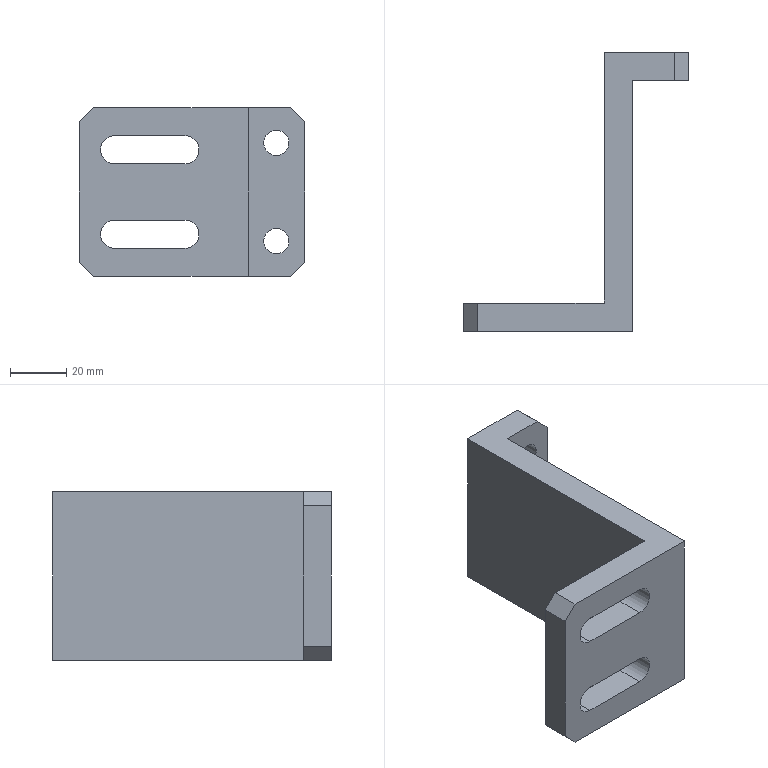Part | SolidWorks | features HoleWzd 2, Chamfer 1, Extrusion 1 | 1 solid | 26 faces | box 80 x 99 x 60 mm | volume 93057 mm3 | plane 18 | cylinder 8 | commonest cylinder face diameters 9 x4 10 x4
STEP:
#1=CARTESIAN_POINT('',(10.,89.,-22.));
#2=VERTEX_POINT('',#1);
#3=CARTESIAN_POINT('',(10.,89.,-13.));
#4=VERTEX_POINT('',#3);
#5=CARTESIAN_POINT('',(10.,89.,-17.5));
#6=DIRECTION('',(0.,1.,0.));
#7=DIRECTION('',(0.,0.,1.));
#8=AXIS2_PLACEMENT_3D('',#5,#6,#7);
#9=CIRCLE('',#8,4.5);
#10=EDGE_CURVE('',#2,#4,#9,.T.);
#11=ORIENTED_EDGE('',*,*,#10,.F.);
#12=CARTESIAN_POINT('',(10.,99.,-22.));
#13=VERTEX_POINT('',#12);
#14=CARTESIAN_POINT('',(10.,99.,-22.));
#15=DIRECTION('',(0.,1.,0.));
#16=VECTOR('',#15,1000.);
#17=LINE('',#14,#16);
#18=EDGE_CURVE('',#2,#13,#17,.T.);
#19=ORIENTED_EDGE('',*,*,#18,.T.);
#20=CARTESIAN_POINT('',(10.,99.,-13.));
#21=VERTEX_POINT('',#20);
#22=CARTESIAN_POINT('',(10.,99.,-17.5));
#23=DIRECTION('',(0.,1.,0.));
#24=DIRECTION('',(0.,0.,1.));
#25=AXIS2_PLACEMENT_3D('',#22,#23,#24);
#26=CIRCLE('',#25,4.5);
#27=EDGE_CURVE('',#13,#21,#26,.T.);
#28=ORIENTED_EDGE('',*,*,#27,.T.);
#29=CARTESIAN_POINT('',(10.,99.,-13.));
#30=DIRECTION('',(0.,1.,0.));
#31=VECTOR('',#30,1000.);
#32=LINE('',#29,#31);
#33=EDGE_CURVE('',#4,#21,#32,.T.);
#34=ORIENTED_EDGE('',*,*,#33,.F.);
#35=EDGE_LOOP('',(#11,#19,#28,#34));
#36=FACE_OUTER_BOUND('',#35,.T.);
#37=CARTESIAN_POINT('',(10.,99.,-17.5));
#38=DIRECTION('',(0.,1.,0.));
#39=DIRECTION('',(0.,0.,1.));
#40=AXIS2_PLACEMENT_3D('',#37,#38,#39);
#41=CYLINDRICAL_SURFACE('',#40,4.5);
#42=ADVANCED_FACE('',(#36),#41,.F.);
#43=CARTESIAN_POINT('',(10.,89.,13.));
#44=VERTEX_POINT('',#43);
#45=CARTESIAN_POINT('',(10.,89.,22.));
#46=VERTEX_POINT('',#45);
#47=CARTESIAN_POINT('',(10.,89.,17.5));
#48=DIRECTION('',(0.,1.,0.));
#49=DIRECTION('',(0.,0.,1.));
#50=AXIS2_PLACEMENT_3D('',#47,#48,#49);
#51=CIRCLE('',#50,4.5);
#52=EDGE_CURVE('',#44,#46,#51,.T.);
#53=ORIENTED_EDGE('',*,*,#52,.F.);
#54=CARTESIAN_POINT('',(10.,99.,13.));
#55=VERTEX_POINT('',#54);
#56=CARTESIAN_POINT('',(10.,99.,13.));
#57=DIRECTION('',(0.,1.,0.));
#58=VECTOR('',#57,1000.);
#59=LINE('',#56,#58);
#60=EDGE_CURVE('',#44,#55,#59,.T.);
#61=ORIENTED_EDGE('',*,*,#60,.T.);
#62=CARTESIAN_POINT('',(10.,99.,22.));
#63=VERTEX_POINT('',#62);
#64=CARTESIAN_POINT('',(10.,99.,17.5));
#65=DIRECTION('',(0.,1.,0.));
#66=DIRECTION('',(0.,0.,1.));
#67=AXIS2_PLACEMENT_3D('',#64,#65,#66);
#68=CIRCLE('',#67,4.5);
#69=EDGE_CURVE('',#55,#63,#68,.T.);
#70=ORIENTED_EDGE('',*,*,#69,.T.);
#71=CARTESIAN_POINT('',(10.,99.,22.));
#72=DIRECTION('',(0.,1.,0.));
#73=VECTOR('',#72,1000.);
#74=LINE('',#71,#73);
#75=EDGE_CURVE('',#46,#63,#74,.T.);
#76=ORIENTED_EDGE('',*,*,#75,.F.);
#77=EDGE_LOOP('',(#53,#61,#70,#76));
#78=FACE_OUTER_BOUND('',#77,.T.);
#79=CARTESIAN_POINT('',(10.,99.,17.5));
#80=DIRECTION('',(0.,1.,0.));
#81=DIRECTION('',(0.,0.,1.));
#82=AXIS2_PLACEMENT_3D('',#79,#80,#81);
#83=CYLINDRICAL_SURFACE('',#82,4.5);
#84=ADVANCED_FACE('',(#78),#83,.F.);
#85=CARTESIAN_POINT('',(10.,99.,17.5));
#86=DIRECTION('',(0.,1.,0.));
#87=DIRECTION('',(0.,0.,1.));
#88=AXIS2_PLACEMENT_3D('',#85,#86,#87);
#89=CIRCLE('',#88,4.5);
#90=EDGE_CURVE('',#63,#55,#89,.T.);
#91=ORIENTED_EDGE('',*,*,#90,.F.);
#92=ORIENTED_EDGE('',*,*,#69,.F.);
#93=EDGE_LOOP('',(#91,#92));
#94=FACE_BOUND('',#93,.T.);
#95=CARTESIAN_POINT('',(20.,99.,25.));
#96=VERTEX_POINT('',#95);
#97=CARTESIAN_POINT('',(20.,99.,-25.));
#98=VERTEX_POINT('',#97);
#99=CARTESIAN_POINT('',(20.,99.,30.));
#100=DIRECTION('',(0.,0.,-1.));
#101=VECTOR('',#100,1000.);
#102=LINE('',#99,#101);
#103=EDGE_CURVE('',#96,#98,#102,.T.);
#104=ORIENTED_EDGE('',*,*,#103,.T.);
#105=CARTESIAN_POINT('',(15.,99.,-30.));
#106=VERTEX_POINT('',#105);
#107=CARTESIAN_POINT('',(20.,99.,-25.));
#108=DIRECTION('',(-0.7071,0.,-0.7071));
#109=VECTOR('',#108,1000.);
#110=LINE('',#107,#109);
#111=EDGE_CURVE('',#98,#106,#110,.T.);
#112=ORIENTED_EDGE('',*,*,#111,.T.);
#113=CARTESIAN_POINT('',(-10.,99.,-30.));
#114=VERTEX_POINT('',#113);
#115=CARTESIAN_POINT('',(-10.,99.,-30.));
#116=DIRECTION('',(-1.,0.,0.));
#117=VECTOR('',#116,1000.);
#118=LINE('',#115,#117);
#119=EDGE_CURVE('',#106,#114,#118,.T.);
#120=ORIENTED_EDGE('',*,*,#119,.T.);
#121=CARTESIAN_POINT('',(-10.,99.,30.));
#122=VERTEX_POINT('',#121);
#123=CARTESIAN_POINT('',(-10.,99.,30.));
#124=DIRECTION('',(0.,0.,-1.));
#125=VECTOR('',#124,1000.);
#126=LINE('',#123,#125);
#127=EDGE_CURVE('',#122,#114,#126,.T.);
#128=ORIENTED_EDGE('',*,*,#127,.F.);
#129=CARTESIAN_POINT('',(15.,99.,30.));
#130=VERTEX_POINT('',#129);
#131=CARTESIAN_POINT('',(-10.,99.,30.));
#132=DIRECTION('',(-1.,0.,0.));
#133=VECTOR('',#132,1000.);
#134=LINE('',#131,#133);
#135=EDGE_CURVE('',#130,#122,#134,.T.);
#136=ORIENTED_EDGE('',*,*,#135,.F.);
#137=CARTESIAN_POINT('',(15.,99.,30.));
#138=DIRECTION('',(0.7071,0.,-0.7071));
#139=VECTOR('',#138,1000.);
#140=LINE('',#137,#139);
#141=EDGE_CURVE('',#130,#96,#140,.T.);
#142=ORIENTED_EDGE('',*,*,#141,.T.);
#143=EDGE_LOOP('',(#104,#112,#120,#128,#136,#142));
#144=FACE_OUTER_BOUND('',#143,.T.);
#145=CARTESIAN_POINT('',(10.,99.,-17.5));
#146=DIRECTION('',(0.,1.,0.));
#147=DIRECTION('',(0.,0.,1.));
#148=AXIS2_PLACEMENT_3D('',#145,#146,#147);
#149=CIRCLE('',#148,4.5);
#150=EDGE_CURVE('',#21,#13,#149,.T.);
#151=ORIENTED_EDGE('',*,*,#150,.F.);
#152=ORIENTED_EDGE('',*,*,#27,.F.);
#153=EDGE_LOOP('',(#151,#152));
#154=FACE_BOUND('',#153,.T.);
#155=CARTESIAN_POINT('',(-10.,99.,30.));
#156=DIRECTION('',(0.,-1.,0.));
#157=DIRECTION('',(0.,0.,-1.));
#158=AXIS2_PLACEMENT_3D('',#155,#156,#157);
#159=PLANE('',#158);
#160=ADVANCED_FACE('',(#94,#144,#154),#159,.F.);
#161=CARTESIAN_POINT('',(-47.5,0.,-10.));
#162=VERTEX_POINT('',#161);
#163=CARTESIAN_POINT('',(-22.5,0.,-10.));
#164=VERTEX_POINT('',#163);
#165=CARTESIAN_POINT('',(-47.5,0.,-10.));
#166=DIRECTION('',(1.,0.,0.));
#167=VECTOR('',#166,1000.);
#168=LINE('',#165,#167);
#169=EDGE_CURVE('',#162,#164,#168,.T.);
#170=ORIENTED_EDGE('',*,*,#169,.T.);
#171=CARTESIAN_POINT('',(-22.5,0.,-20.));
#172=VERTEX_POINT('',#171);
#173=CARTESIAN_POINT('',(-22.5,0.,-15.));
#174=DIRECTION('',(0.,1.,0.));
#175=DIRECTION('',(0.,0.,1.));
#176=AXIS2_PLACEMENT_3D('',#173,#174,#175);
#177=CIRCLE('',#176,5.);
#178=EDGE_CURVE('',#164,#172,#177,.T.);
#179=ORIENTED_EDGE('',*,*,#178,.T.);
#180=CARTESIAN_POINT('',(-47.5,0.,-20.));
#181=VERTEX_POINT('',#180);
#182=CARTESIAN_POINT('',(-47.5,0.,-20.));
#183=DIRECTION('',(1.,0.,0.));
#184=VECTOR('',#183,1000.);
#185=LINE('',#182,#184);
#186=EDGE_CURVE('',#181,#172,#185,.T.);
#187=ORIENTED_EDGE('',*,*,#186,.F.);
#188=CARTESIAN_POINT('',(-47.5,0.,-15.));
#189=DIRECTION('',(0.,1.,0.));
#190=DIRECTION('',(0.,0.,1.));
#191=AXIS2_PLACEMENT_3D('',#188,#189,#190);
#192=CIRCLE('',#191,5.);
#193=EDGE_CURVE('',#181,#162,#192,.T.);
#194=ORIENTED_EDGE('',*,*,#193,.T.);
#195=EDGE_LOOP('',(#170,#179,#187,#194));
#196=FACE_BOUND('',#195,.T.);
#197=CARTESIAN_POINT('',(-47.5,0.,20.));
#198=VERTEX_POINT('',#197);
#199=CARTESIAN_POINT('',(-22.5,0.,20.));
#200=VERTEX_POINT('',#199);
#201=CARTESIAN_POINT('',(-47.5,0.,20.));
#202=DIRECTION('',(1.,0.,0.));
#203=VECTOR('',#202,1000.);
#204=LINE('',#201,#203);
#205=EDGE_CURVE('',#198,#200,#204,.T.);
#206=ORIENTED_EDGE('',*,*,#205,.T.);
#207=CARTESIAN_POINT('',(-22.5,0.,10.));
#208=VERTEX_POINT('',#207);
#209=CARTESIAN_POINT('',(-22.5,0.,15.));
#210=DIRECTION('',(0.,1.,0.));
#211=DIRECTION('',(0.,0.,1.));
#212=AXIS2_PLACEMENT_3D('',#209,#210,#211);
#213=CIRCLE('',#212,5.);
#214=EDGE_CURVE('',#200,#208,#213,.T.);
#215=ORIENTED_EDGE('',*,*,#214,.T.);
#216=CARTESIAN_POINT('',(-47.5,0.,10.));
#217=VERTEX_POINT('',#216);
#218=CARTESIAN_POINT('',(-47.5,0.,10.));
#219=DIRECTION('',(1.,0.,0.));
#220=VECTOR('',#219,1000.);
#221=LINE('',#218,#220);
#222=EDGE_CURVE('',#217,#208,#221,.T.);
#223=ORIENTED_EDGE('',*,*,#222,.F.);
#224=CARTESIAN_POINT('',(-47.5,0.,15.));
#225=DIRECTION('',(0.,1.,0.));
#226=DIRECTION('',(0.,0.,1.));
#227=AXIS2_PLACEMENT_3D('',#224,#225,#226);
#228=CIRCLE('',#227,5.);
#229=EDGE_CURVE('',#217,#198,#228,.T.);
#230=ORIENTED_EDGE('',*,*,#229,.T.);
#231=EDGE_LOOP('',(#206,#215,#223,#230));
#232=FACE_BOUND('',#231,.T.);
#233=CARTESIAN_POINT('',(-60.,0.,25.));
#234=VERTEX_POINT('',#233);
#235=CARTESIAN_POINT('',(-60.,0.,-25.));
#236=VERTEX_POINT('',#235);
#237=CARTESIAN_POINT('',(-60.,0.,30.));
#238=DIRECTION('',(0.,0.,-1.));
#239=VECTOR('',#238,1000.);
#240=LINE('',#237,#239);
#241=EDGE_CURVE('',#234,#236,#240,.T.);
#242=ORIENTED_EDGE('',*,*,#241,.T.);
#243=CARTESIAN_POINT('',(-55.,0.,-30.));
#244=VERTEX_POINT('',#243);
#245=CARTESIAN_POINT('',(-60.,0.,-25.));
#246=DIRECTION('',(0.7071,0.,-0.7071));
#247=VECTOR('',#246,1000.);
#248=LINE('',#245,#247);
#249=EDGE_CURVE('',#236,#244,#248,.T.);
#250=ORIENTED_EDGE('',*,*,#249,.T.);
#251=CARTESIAN_POINT('',(0.,0.,-30.));
#252=VERTEX_POINT('',#251);
#253=CARTESIAN_POINT('',(0.,0.,-30.));
#254=DIRECTION('',(1.,0.,0.));
#255=VECTOR('',#254,1000.);
#256=LINE('',#253,#255);
#257=EDGE_CURVE('',#244,#252,#256,.T.);
#258=ORIENTED_EDGE('',*,*,#257,.T.);
#259=CARTESIAN_POINT('',(0.,0.,30.));
#260=VERTEX_POINT('',#259);
#261=CARTESIAN_POINT('',(0.,0.,30.));
#262=DIRECTION('',(0.,0.,-1.));
#263=VECTOR('',#262,1000.);
#264=LINE('',#261,#263);
#265=EDGE_CURVE('',#260,#252,#264,.T.);
#266=ORIENTED_EDGE('',*,*,#265,.F.);
#267=CARTESIAN_POINT('',(-55.,0.,30.));
#268=VERTEX_POINT('',#267);
#269=CARTESIAN_POINT('',(0.,0.,30.));
#270=DIRECTION('',(1.,0.,0.));
#271=VECTOR('',#270,1000.);
#272=LINE('',#269,#271);
#273=EDGE_CURVE('',#268,#260,#272,.T.);
#274=ORIENTED_EDGE('',*,*,#273,.F.);
#275=CARTESIAN_POINT('',(-55.,0.,30.));
#276=DIRECTION('',(-0.7071,0.,-0.7071));
#277=VECTOR('',#276,1000.);
#278=LINE('',#275,#277);
#279=EDGE_CURVE('',#268,#234,#278,.T.);
#280=ORIENTED_EDGE('',*,*,#279,.T.);
#281=EDGE_LOOP('',(#242,#250,#258,#266,#274,#280));
#282=FACE_OUTER_BOUND('',#281,.T.);
#283=CARTESIAN_POINT('',(0.,0.,30.));
#284=DIRECTION('',(0.,1.,0.));
#285=DIRECTION('',(-1.,0.,0.));
#286=AXIS2_PLACEMENT_3D('',#283,#284,#285);
#287=PLANE('',#286);
#288=ADVANCED_FACE('',(#196,#232,#282),#287,.F.);
#289=CARTESIAN_POINT('',(0.,89.,-30.));
#290=VERTEX_POINT('',#289);
#291=CARTESIAN_POINT('',(0.,0.,-30.));
#292=DIRECTION('',(0.,1.,0.));
#293=VECTOR('',#292,1000.);
#294=LINE('',#291,#293);
#295=EDGE_CURVE('',#252,#290,#294,.T.);
#296=ORIENTED_EDGE('',*,*,#295,.T.);
#297=CARTESIAN_POINT('',(0.,89.,30.));
#298=VERTEX_POINT('',#297);
#299=CARTESIAN_POINT('',(0.,89.,30.));
#300=DIRECTION('',(0.,0.,-1.));
#301=VECTOR('',#300,1000.);
#302=LINE('',#299,#301);
#303=EDGE_CURVE('',#298,#290,#302,.T.);
#304=ORIENTED_EDGE('',*,*,#303,.F.);
#305=CARTESIAN_POINT('',(0.,0.,30.));
#306=DIRECTION('',(0.,1.,0.));
#307=VECTOR('',#306,1000.);
#308=LINE('',#305,#307);
#309=EDGE_CURVE('',#260,#298,#308,.T.);
#310=ORIENTED_EDGE('',*,*,#309,.F.);
#311=ORIENTED_EDGE('',*,*,#265,.T.);
#312=EDGE_LOOP('',(#296,#304,#310,#311));
#313=FACE_OUTER_BOUND('',#312,.T.);
#314=CARTESIAN_POINT('',(0.,0.,30.));
#315=DIRECTION('',(-1.,0.,0.));
#316=DIRECTION('',(0.,0.,1.));
#317=AXIS2_PLACEMENT_3D('',#314,#315,#316);
#318=PLANE('',#317);
#319=ADVANCED_FACE('',(#313),#318,.F.);
#320=CARTESIAN_POINT('',(10.,89.,-17.5));
#321=DIRECTION('',(0.,1.,0.));
#322=DIRECTION('',(0.,0.,1.));
#323=AXIS2_PLACEMENT_3D('',#320,#321,#322);
#324=CIRCLE('',#323,4.5);
#325=EDGE_CURVE('',#4,#2,#324,.T.);
#326=ORIENTED_EDGE('',*,*,#325,.T.);
#327=ORIENTED_EDGE('',*,*,#10,.T.);
#328=EDGE_LOOP('',(#326,#327));
#329=FACE_BOUND('',#328,.T.);
#330=CARTESIAN_POINT('',(10.,89.,17.5));
#331=DIRECTION('',(0.,1.,0.));
#332=DIRECTION('',(0.,0.,1.));
#333=AXIS2_PLACEMENT_3D('',#330,#331,#332);
#334=CIRCLE('',#333,4.5);
#335=EDGE_CURVE('',#46,#44,#334,.T.);
#336=ORIENTED_EDGE('',*,*,#335,.T.);
#337=ORIENTED_EDGE('',*,*,#52,.T.);
#338=EDGE_LOOP('',(#336,#337));
#339=FACE_BOUND('',#338,.T.);
#340=CARTESIAN_POINT('',(15.,89.,-30.));
#341=VERTEX_POINT('',#340);
#342=CARTESIAN_POINT('',(0.,89.,-30.));
#343=DIRECTION('',(1.,0.,0.));
#344=VECTOR('',#343,1000.);
#345=LINE('',#342,#344);
#346=EDGE_CURVE('',#290,#341,#345,.T.);
#347=ORIENTED_EDGE('',*,*,#346,.T.);
#348=CARTESIAN_POINT('',(20.,89.,-25.));
#349=VERTEX_POINT('',#348);
#350=CARTESIAN_POINT('',(20.,89.,-25.));
#351=DIRECTION('',(0.7071,0.,0.7071));
#352=VECTOR('',#351,1000.);
#353=LINE('',#350,#352);
#354=EDGE_CURVE('',#341,#349,#353,.T.);
#355=ORIENTED_EDGE('',*,*,#354,.T.);
#356=CARTESIAN_POINT('',(20.,89.,25.));
#357=VERTEX_POINT('',#356);
#358=CARTESIAN_POINT('',(20.,89.,30.));
#359=DIRECTION('',(0.,0.,-1.));
#360=VECTOR('',#359,1000.);
#361=LINE('',#358,#360);
#362=EDGE_CURVE('',#357,#349,#361,.T.);
#363=ORIENTED_EDGE('',*,*,#362,.F.);
#364=CARTESIAN_POINT('',(15.,89.,30.));
#365=VERTEX_POINT('',#364);
#366=CARTESIAN_POINT('',(15.,89.,30.));
#367=DIRECTION('',(-0.7071,0.,0.7071));
#368=VECTOR('',#367,1000.);
#369=LINE('',#366,#368);
#370=EDGE_CURVE('',#357,#365,#369,.T.);
#371=ORIENTED_EDGE('',*,*,#370,.T.);
#372=CARTESIAN_POINT('',(0.,89.,30.));
#373=DIRECTION('',(1.,0.,0.));
#374=VECTOR('',#373,1000.);
#375=LINE('',#372,#374);
#376=EDGE_CURVE('',#298,#365,#375,.T.);
#377=ORIENTED_EDGE('',*,*,#376,.F.);
#378=ORIENTED_EDGE('',*,*,#303,.T.);
#379=EDGE_LOOP('',(#347,#355,#363,#371,#377,#378));
#380=FACE_OUTER_BOUND('',#379,.T.);
#381=CARTESIAN_POINT('',(0.,89.,30.));
#382=DIRECTION('',(0.,1.,0.));
#383=DIRECTION('',(0.,0.,1.));
#384=AXIS2_PLACEMENT_3D('',#381,#382,#383);
#385=PLANE('',#384);
#386=ADVANCED_FACE('',(#329,#339,#380),#385,.F.);
#387=ORIENTED_EDGE('',*,*,#362,.T.);
#388=CARTESIAN_POINT('',(20.,99.,-25.));
#389=DIRECTION('',(0.,1.,0.));
#390=VECTOR('',#389,1000.);
#391=LINE('',#388,#390);
#392=EDGE_CURVE('',#349,#98,#391,.T.);
#393=ORIENTED_EDGE('',*,*,#392,.T.);
#394=ORIENTED_EDGE('',*,*,#103,.F.);
#395=CARTESIAN_POINT('',(20.,89.,25.));
#396=DIRECTION('',(0.,-1.,0.));
#397=VECTOR('',#396,1000.);
#398=LINE('',#395,#397);
#399=EDGE_CURVE('',#96,#357,#398,.T.);
#400=ORIENTED_EDGE('',*,*,#399,.T.);
#401=EDGE_LOOP('',(#387,#393,#394,#400));
#402=FACE_OUTER_BOUND('',#401,.T.);
#403=CARTESIAN_POINT('',(20.,99.,30.));
#404=DIRECTION('',(-1.,0.,0.));
#405=DIRECTION('',(0.,0.,1.));
#406=AXIS2_PLACEMENT_3D('',#403,#404,#405);
#407=PLANE('',#406);
#408=ADVANCED_FACE('',(#402),#407,.F.);
#409=CARTESIAN_POINT('',(-10.,10.,-30.));
#410=VERTEX_POINT('',#409);
#411=CARTESIAN_POINT('',(-10.,10.,-30.));
#412=DIRECTION('',(0.,-1.,0.));
#413=VECTOR('',#412,1000.);
#414=LINE('',#411,#413);
#415=EDGE_CURVE('',#114,#410,#414,.T.);
#416=ORIENTED_EDGE('',*,*,#415,.T.);
#417=CARTESIAN_POINT('',(-10.,10.,30.));
#418=VERTEX_POINT('',#417);
#419=CARTESIAN_POINT('',(-10.,10.,30.));
#420=DIRECTION('',(0.,0.,-1.));
#421=VECTOR('',#420,1000.);
#422=LINE('',#419,#421);
#423=EDGE_CURVE('',#418,#410,#422,.T.);
#424=ORIENTED_EDGE('',*,*,#423,.F.);
#425=CARTESIAN_POINT('',(-10.,10.,30.));
#426=DIRECTION('',(0.,-1.,0.));
#427=VECTOR('',#426,1000.);
#428=LINE('',#425,#427);
#429=EDGE_CURVE('',#122,#418,#428,.T.);
#430=ORIENTED_EDGE('',*,*,#429,.F.);
#431=ORIENTED_EDGE('',*,*,#127,.T.);
#432=EDGE_LOOP('',(#416,#424,#430,#431));
#433=FACE_OUTER_BOUND('',#432,.T.);
#434=CARTESIAN_POINT('',(-10.,10.,30.));
#435=DIRECTION('',(1.,0.,0.));
#436=DIRECTION('',(0.,0.,-1.));
#437=AXIS2_PLACEMENT_3D('',#434,#435,#436);
#438=PLANE('',#437);
#439=ADVANCED_FACE('',(#433),#438,.F.);
#440=CARTESIAN_POINT('',(-47.5,10.,-20.));
#441=VERTEX_POINT('',#440);
#442=CARTESIAN_POINT('',(-47.5,10.,-10.));
#443=VERTEX_POINT('',#442);
#444=CARTESIAN_POINT('',(-47.5,10.,-15.));
#445=DIRECTION('',(0.,1.,0.));
#446=DIRECTION('',(0.,0.,1.));
#447=AXIS2_PLACEMENT_3D('',#444,#445,#446);
#448=CIRCLE('',#447,5.);
#449=EDGE_CURVE('',#441,#443,#448,.T.);
#450=ORIENTED_EDGE('',*,*,#449,.F.);
#451=CARTESIAN_POINT('',(-22.5,10.,-20.));
#452=VERTEX_POINT('',#451);
#453=CARTESIAN_POINT('',(-47.5,10.,-20.));
#454=DIRECTION('',(1.,0.,0.));
#455=VECTOR('',#454,1000.);
#456=LINE('',#453,#455);
#457=EDGE_CURVE('',#441,#452,#456,.T.);
#458=ORIENTED_EDGE('',*,*,#457,.T.);
#459=CARTESIAN_POINT('',(-22.5,10.,-10.));
#460=VERTEX_POINT('',#459);
#461=CARTESIAN_POINT('',(-22.5,10.,-15.));
#462=DIRECTION('',(0.,1.,0.));
#463=DIRECTION('',(0.,0.,1.));
#464=AXIS2_PLACEMENT_3D('',#461,#462,#463);
#465=CIRCLE('',#464,5.);
#466=EDGE_CURVE('',#460,#452,#465,.T.);
#467=ORIENTED_EDGE('',*,*,#466,.F.);
#468=CARTESIAN_POINT('',(-47.5,10.,-10.));
#469=DIRECTION('',(1.,0.,0.));
#470=VECTOR('',#469,1000.);
#471=LINE('',#468,#470);
#472=EDGE_CURVE('',#443,#460,#471,.T.);
#473=ORIENTED_EDGE('',*,*,#472,.F.);
#474=EDGE_LOOP('',(#450,#458,#467,#473));
#475=FACE_BOUND('',#474,.T.);
#476=CARTESIAN_POINT('',(-47.5,10.,10.));
#477=VERTEX_POINT('',#476);
#478=CARTESIAN_POINT('',(-47.5,10.,20.));
#479=VERTEX_POINT('',#478);
#480=CARTESIAN_POINT('',(-47.5,10.,15.));
#481=DIRECTION('',(0.,1.,0.));
#482=DIRECTION('',(0.,0.,1.));
#483=AXIS2_PLACEMENT_3D('',#480,#481,#482);
#484=CIRCLE('',#483,5.);
#485=EDGE_CURVE('',#477,#479,#484,.T.);
#486=ORIENTED_EDGE('',*,*,#485,.F.);
#487=CARTESIAN_POINT('',(-22.5,10.,10.));
#488=VERTEX_POINT('',#487);
#489=CARTESIAN_POINT('',(-47.5,10.,10.));
#490=DIRECTION('',(1.,0.,0.));
#491=VECTOR('',#490,1000.);
#492=LINE('',#489,#491);
#493=EDGE_CURVE('',#477,#488,#492,.T.);
#494=ORIENTED_EDGE('',*,*,#493,.T.);
#495=CARTESIAN_POINT('',(-22.5,10.,20.));
#496=VERTEX_POINT('',#495);
#497=CARTESIAN_POINT('',(-22.5,10.,15.));
#498=DIRECTION('',(0.,1.,0.));
#499=DIRECTION('',(0.,0.,1.));
#500=AXIS2_PLACEMENT_3D('',#497,#498,#499);
#501=CIRCLE('',#500,5.);
#502=EDGE_CURVE('',#496,#488,#501,.T.);
#503=ORIENTED_EDGE('',*,*,#502,.F.);
#504=CARTESIAN_POINT('',(-47.5,10.,20.));
#505=DIRECTION('',(1.,0.,0.));
#506=VECTOR('',#505,1000.);
#507=LINE('',#504,#506);
#508=EDGE_CURVE('',#479,#496,#507,.T.);
#509=ORIENTED_EDGE('',*,*,#508,.F.);
#510=EDGE_LOOP('',(#486,#494,#503,#509));
#511=FACE_BOUND('',#510,.T.);
#512=CARTESIAN_POINT('',(-55.,10.,-30.));
#513=VERTEX_POINT('',#512);
#514=CARTESIAN_POINT('',(-10.,10.,-30.));
#515=DIRECTION('',(-1.,0.,0.));
#516=VECTOR('',#515,1000.);
#517=LINE('',#514,#516);
#518=EDGE_CURVE('',#410,#513,#517,.T.);
#519=ORIENTED_EDGE('',*,*,#518,.T.);
#520=CARTESIAN_POINT('',(-60.,10.,-25.));
#521=VERTEX_POINT('',#520);
#522=CARTESIAN_POINT('',(-60.,10.,-25.));
#523=DIRECTION('',(-0.7071,0.,0.7071));
#524=VECTOR('',#523,1000.);
#525=LINE('',#522,#524);
#526=EDGE_CURVE('',#513,#521,#525,.T.);
#527=ORIENTED_EDGE('',*,*,#526,.T.);
#528=CARTESIAN_POINT('',(-60.,10.,25.));
#529=VERTEX_POINT('',#528);
#530=CARTESIAN_POINT('',(-60.,10.,30.));
#531=DIRECTION('',(0.,0.,-1.));
#532=VECTOR('',#531,1000.);
#533=LINE('',#530,#532);
#534=EDGE_CURVE('',#529,#521,#533,.T.);
#535=ORIENTED_EDGE('',*,*,#534,.F.);
#536=CARTESIAN_POINT('',(-55.,10.,30.));
#537=VERTEX_POINT('',#536);
#538=CARTESIAN_POINT('',(-55.,10.,30.));
#539=DIRECTION('',(0.7071,0.,0.7071));
#540=VECTOR('',#539,1000.);
#541=LINE('',#538,#540);
#542=EDGE_CURVE('',#529,#537,#541,.T.);
#543=ORIENTED_EDGE('',*,*,#542,.T.);
#544=CARTESIAN_POINT('',(-10.,10.,30.));
#545=DIRECTION('',(-1.,0.,0.));
#546=VECTOR('',#545,1000.);
#547=LINE('',#544,#546);
#548=EDGE_CURVE('',#418,#537,#547,.T.);
#549=ORIENTED_EDGE('',*,*,#548,.F.);
#550=ORIENTED_EDGE('',*,*,#423,.T.);
#551=EDGE_LOOP('',(#519,#527,#535,#543,#549,#550));
#552=FACE_OUTER_BOUND('',#551,.T.);
#553=CARTESIAN_POINT('',(-10.,10.,30.));
#554=DIRECTION('',(0.,-1.,0.));
#555=DIRECTION('',(1.,0.,0.));
#556=AXIS2_PLACEMENT_3D('',#553,#554,#555);
#557=PLANE('',#556);
#558=ADVANCED_FACE('',(#475,#511,#552),#557,.F.);
#559=ORIENTED_EDGE('',*,*,#534,.T.);
#560=CARTESIAN_POINT('',(-60.,10.,-25.));
#561=DIRECTION('',(0.,-1.,0.));
#562=VECTOR('',#561,1000.);
#563=LINE('',#560,#562);
#564=EDGE_CURVE('',#521,#236,#563,.T.);
#565=ORIENTED_EDGE('',*,*,#564,.T.);
#566=ORIENTED_EDGE('',*,*,#241,.F.);
#567=CARTESIAN_POINT('',(-60.,10.,25.));
#568=DIRECTION('',(0.,1.,0.));
#569=VECTOR('',#568,1000.);
#570=LINE('',#567,#569);
#571=EDGE_CURVE('',#234,#529,#570,.T.);
#572=ORIENTED_EDGE('',*,*,#571,.T.);
#573=EDGE_LOOP('',(#559,#565,#566,#572));
#574=FACE_OUTER_BOUND('',#573,.T.);
#575=CARTESIAN_POINT('',(-60.,10.,30.));
#576=DIRECTION('',(1.,0.,0.));
#577=DIRECTION('',(0.,0.,-1.));
#578=AXIS2_PLACEMENT_3D('',#575,#576,#577);
#579=PLANE('',#578);
#580=ADVANCED_FACE('',(#574),#579,.F.);
#581=ORIENTED_EDGE('',*,*,#548,.T.);
#582=CARTESIAN_POINT('',(-55.,0.,30.));
#583=DIRECTION('',(0.,-1.,0.));
#584=VECTOR('',#583,1000.);
#585=LINE('',#582,#584);
#586=EDGE_CURVE('',#537,#268,#585,.T.);
#587=ORIENTED_EDGE('',*,*,#586,.T.);
#588=ORIENTED_EDGE('',*,*,#273,.T.);
#589=ORIENTED_EDGE('',*,*,#309,.T.);
#590=ORIENTED_EDGE('',*,*,#376,.T.);
#591=CARTESIAN_POINT('',(15.,99.,30.));
#592=DIRECTION('',(0.,1.,0.));
#593=VECTOR('',#592,1000.);
#594=LINE('',#591,#593);
#595=EDGE_CURVE('',#365,#130,#594,.T.);
#596=ORIENTED_EDGE('',*,*,#595,.T.);
#597=ORIENTED_EDGE('',*,*,#135,.T.);
#598=ORIENTED_EDGE('',*,*,#429,.T.);
#599=EDGE_LOOP('',(#581,#587,#588,#589,#590,#596,#597,#598));
#600=FACE_OUTER_BOUND('',#599,.T.);
#601=CARTESIAN_POINT('',(0.,0.,30.));
#602=DIRECTION('',(0.,0.,1.));
#603=DIRECTION('',(1.,0.,0.));
#604=AXIS2_PLACEMENT_3D('',#601,#602,#603);
#605=PLANE('',#604);
#606=ADVANCED_FACE('',(#600),#605,.T.);
#607=ORIENTED_EDGE('',*,*,#257,.F.);
#608=CARTESIAN_POINT('',(-55.,0.,-30.));
#609=DIRECTION('',(0.,1.,0.));
#610=VECTOR('',#609,1000.);
#611=LINE('',#608,#610);
#612=EDGE_CURVE('',#244,#513,#611,.T.);
#613=ORIENTED_EDGE('',*,*,#612,.T.);
#614=ORIENTED_EDGE('',*,*,#518,.F.);
#615=ORIENTED_EDGE('',*,*,#415,.F.);
#616=ORIENTED_EDGE('',*,*,#119,.F.);
#617=CARTESIAN_POINT('',(15.,0.,-30.));
#618=DIRECTION('',(0.,-1.,0.));
#619=VECTOR('',#618,1000.);
#620=LINE('',#617,#619);
#621=EDGE_CURVE('',#106,#341,#620,.T.);
#622=ORIENTED_EDGE('',*,*,#621,.T.);
#623=ORIENTED_EDGE('',*,*,#346,.F.);
#624=ORIENTED_EDGE('',*,*,#295,.F.);
#625=EDGE_LOOP('',(#607,#613,#614,#615,#616,#622,#623,#624));
#626=FACE_OUTER_BOUND('',#625,.T.);
#627=CARTESIAN_POINT('',(0.,0.,-30.));
#628=DIRECTION('',(0.,0.,1.));
#629=DIRECTION('',(1.,0.,0.));
#630=AXIS2_PLACEMENT_3D('',#627,#628,#629);
#631=PLANE('',#630);
#632=ADVANCED_FACE('',(#626),#631,.F.);
#633=ORIENTED_EDGE('',*,*,#60,.F.);
#634=ORIENTED_EDGE('',*,*,#335,.F.);
#635=ORIENTED_EDGE('',*,*,#75,.T.);
#636=ORIENTED_EDGE('',*,*,#90,.T.);
#637=EDGE_LOOP('',(#633,#634,#635,#636));
#638=FACE_OUTER_BOUND('',#637,.T.);
#639=CARTESIAN_POINT('',(10.,99.,17.5));
#640=DIRECTION('',(0.,1.,0.));
#641=DIRECTION('',(0.,0.,1.));
#642=AXIS2_PLACEMENT_3D('',#639,#640,#641);
#643=CYLINDRICAL_SURFACE('',#642,4.5);
#644=ADVANCED_FACE('',(#638),#643,.F.);
#645=ORIENTED_EDGE('',*,*,#18,.F.);
#646=ORIENTED_EDGE('',*,*,#325,.F.);
#647=ORIENTED_EDGE('',*,*,#33,.T.);
#648=ORIENTED_EDGE('',*,*,#150,.T.);
#649=EDGE_LOOP('',(#645,#646,#647,#648));
#650=FACE_OUTER_BOUND('',#649,.T.);
#651=CARTESIAN_POINT('',(10.,99.,-17.5));
#652=DIRECTION('',(0.,1.,0.));
#653=DIRECTION('',(0.,0.,1.));
#654=AXIS2_PLACEMENT_3D('',#651,#652,#653);
#655=CYLINDRICAL_SURFACE('',#654,4.5);
#656=ADVANCED_FACE('',(#650),#655,.F.);
#657=ORIENTED_EDGE('',*,*,#214,.F.);
#658=CARTESIAN_POINT('',(-22.5,10.,20.));
#659=DIRECTION('',(0.,-1.,0.));
#660=VECTOR('',#659,1000.);
#661=LINE('',#658,#660);
#662=EDGE_CURVE('',#496,#200,#661,.T.);
#663=ORIENTED_EDGE('',*,*,#662,.F.);
#664=ORIENTED_EDGE('',*,*,#502,.T.);
#665=CARTESIAN_POINT('',(-22.5,10.,10.));
#666=DIRECTION('',(0.,1.,0.));
#667=VECTOR('',#666,1000.);
#668=LINE('',#665,#667);
#669=EDGE_CURVE('',#208,#488,#668,.T.);
#670=ORIENTED_EDGE('',*,*,#669,.F.);
#671=EDGE_LOOP('',(#657,#663,#664,#670));
#672=FACE_OUTER_BOUND('',#671,.T.);
#673=CARTESIAN_POINT('',(-22.5,10.,15.));
#674=DIRECTION('',(0.,1.,0.));
#675=DIRECTION('',(0.,0.,1.));
#676=AXIS2_PLACEMENT_3D('',#673,#674,#675);
#677=CYLINDRICAL_SURFACE('',#676,5.);
#678=ADVANCED_FACE('',(#672),#677,.F.);
#679=ORIENTED_EDGE('',*,*,#485,.T.);
#680=CARTESIAN_POINT('',(-47.5,10.,20.));
#681=DIRECTION('',(0.,1.,0.));
#682=VECTOR('',#681,1000.);
#683=LINE('',#680,#682);
#684=EDGE_CURVE('',#198,#479,#683,.T.);
#685=ORIENTED_EDGE('',*,*,#684,.F.);
#686=ORIENTED_EDGE('',*,*,#229,.F.);
#687=CARTESIAN_POINT('',(-47.5,10.,10.));
#688=DIRECTION('',(0.,-1.,0.));
#689=VECTOR('',#688,1000.);
#690=LINE('',#687,#689);
#691=EDGE_CURVE('',#477,#217,#690,.T.);
#692=ORIENTED_EDGE('',*,*,#691,.F.);
#693=EDGE_LOOP('',(#679,#685,#686,#692));
#694=FACE_OUTER_BOUND('',#693,.T.);
#695=CARTESIAN_POINT('',(-47.5,10.,15.));
#696=DIRECTION('',(0.,1.,0.));
#697=DIRECTION('',(0.,0.,1.));
#698=AXIS2_PLACEMENT_3D('',#695,#696,#697);
#699=CYLINDRICAL_SURFACE('',#698,5.);
#700=ADVANCED_FACE('',(#694),#699,.F.);
#701=ORIENTED_EDGE('',*,*,#669,.T.);
#702=ORIENTED_EDGE('',*,*,#493,.F.);
#703=ORIENTED_EDGE('',*,*,#691,.T.);
#704=ORIENTED_EDGE('',*,*,#222,.T.);
#705=EDGE_LOOP('',(#701,#702,#703,#704));
#706=FACE_OUTER_BOUND('',#705,.T.);
#707=CARTESIAN_POINT('',(-47.5,10.,10.));
#708=DIRECTION('',(0.,0.,-1.));
#709=DIRECTION('',(-1.,0.,0.));
#710=AXIS2_PLACEMENT_3D('',#707,#708,#709);
#711=PLANE('',#710);
#712=ADVANCED_FACE('',(#706),#711,.F.);
#713=ORIENTED_EDGE('',*,*,#662,.T.);
#714=ORIENTED_EDGE('',*,*,#205,.F.);
#715=ORIENTED_EDGE('',*,*,#684,.T.);
#716=ORIENTED_EDGE('',*,*,#508,.T.);
#717=EDGE_LOOP('',(#713,#714,#715,#716));
#718=FACE_OUTER_BOUND('',#717,.T.);
#719=CARTESIAN_POINT('',(-47.5,10.,20.));
#720=DIRECTION('',(0.,0.,1.));
#721=DIRECTION('',(1.,0.,0.));
#722=AXIS2_PLACEMENT_3D('',#719,#720,#721);
#723=PLANE('',#722);
#724=ADVANCED_FACE('',(#718),#723,.F.);
#725=ORIENTED_EDGE('',*,*,#178,.F.);
#726=CARTESIAN_POINT('',(-22.5,10.,-10.));
#727=DIRECTION('',(0.,-1.,0.));
#728=VECTOR('',#727,1000.);
#729=LINE('',#726,#728);
#730=EDGE_CURVE('',#460,#164,#729,.T.);
#731=ORIENTED_EDGE('',*,*,#730,.F.);
#732=ORIENTED_EDGE('',*,*,#466,.T.);
#733=CARTESIAN_POINT('',(-22.5,10.,-20.));
#734=DIRECTION('',(0.,1.,0.));
#735=VECTOR('',#734,1000.);
#736=LINE('',#733,#735);
#737=EDGE_CURVE('',#172,#452,#736,.T.);
#738=ORIENTED_EDGE('',*,*,#737,.F.);
#739=EDGE_LOOP('',(#725,#731,#732,#738));
#740=FACE_OUTER_BOUND('',#739,.T.);
#741=CARTESIAN_POINT('',(-22.5,10.,-15.));
#742=DIRECTION('',(0.,1.,0.));
#743=DIRECTION('',(0.,0.,1.));
#744=AXIS2_PLACEMENT_3D('',#741,#742,#743);
#745=CYLINDRICAL_SURFACE('',#744,5.);
#746=ADVANCED_FACE('',(#740),#745,.F.);
#747=ORIENTED_EDGE('',*,*,#449,.T.);
#748=CARTESIAN_POINT('',(-47.5,10.,-10.));
#749=DIRECTION('',(0.,1.,0.));
#750=VECTOR('',#749,1000.);
#751=LINE('',#748,#750);
#752=EDGE_CURVE('',#162,#443,#751,.T.);
#753=ORIENTED_EDGE('',*,*,#752,.F.);
#754=ORIENTED_EDGE('',*,*,#193,.F.);
#755=CARTESIAN_POINT('',(-47.5,10.,-20.));
#756=DIRECTION('',(0.,-1.,0.));
#757=VECTOR('',#756,1000.);
#758=LINE('',#755,#757);
#759=EDGE_CURVE('',#441,#181,#758,.T.);
#760=ORIENTED_EDGE('',*,*,#759,.F.);
#761=EDGE_LOOP('',(#747,#753,#754,#760));
#762=FACE_OUTER_BOUND('',#761,.T.);
#763=CARTESIAN_POINT('',(-47.5,10.,-15.));
#764=DIRECTION('',(0.,1.,0.));
#765=DIRECTION('',(0.,0.,1.));
#766=AXIS2_PLACEMENT_3D('',#763,#764,#765);
#767=CYLINDRICAL_SURFACE('',#766,5.);
#768=ADVANCED_FACE('',(#762),#767,.F.);
#769=ORIENTED_EDGE('',*,*,#737,.T.);
#770=ORIENTED_EDGE('',*,*,#457,.F.);
#771=ORIENTED_EDGE('',*,*,#759,.T.);
#772=ORIENTED_EDGE('',*,*,#186,.T.);
#773=EDGE_LOOP('',(#769,#770,#771,#772));
#774=FACE_OUTER_BOUND('',#773,.T.);
#775=CARTESIAN_POINT('',(-47.5,10.,-20.));
#776=DIRECTION('',(0.,0.,-1.));
#777=DIRECTION('',(-1.,0.,0.));
#778=AXIS2_PLACEMENT_3D('',#775,#776,#777);
#779=PLANE('',#778);
#780=ADVANCED_FACE('',(#774),#779,.F.);
#781=ORIENTED_EDGE('',*,*,#730,.T.);
#782=ORIENTED_EDGE('',*,*,#169,.F.);
#783=ORIENTED_EDGE('',*,*,#752,.T.);
#784=ORIENTED_EDGE('',*,*,#472,.T.);
#785=EDGE_LOOP('',(#781,#782,#783,#784));
#786=FACE_OUTER_BOUND('',#785,.T.);
#787=CARTESIAN_POINT('',(-47.5,10.,-10.));
#788=DIRECTION('',(0.,0.,1.));
#789=DIRECTION('',(1.,0.,0.));
#790=AXIS2_PLACEMENT_3D('',#787,#788,#789);
#791=PLANE('',#790);
#792=ADVANCED_FACE('',(#786),#791,.F.);
#793=ORIENTED_EDGE('',*,*,#526,.F.);
#794=ORIENTED_EDGE('',*,*,#612,.F.);
#795=ORIENTED_EDGE('',*,*,#249,.F.);
#796=ORIENTED_EDGE('',*,*,#564,.F.);
#797=EDGE_LOOP('',(#793,#794,#795,#796));
#798=FACE_OUTER_BOUND('',#797,.T.);
#799=CARTESIAN_POINT('',(-60.,10.,-25.));
#800=DIRECTION('',(0.7071,0.,0.7071));
#801=DIRECTION('',(0.,-1.,0.));
#802=AXIS2_PLACEMENT_3D('',#799,#800,#801);
#803=PLANE('',#802);
#804=ADVANCED_FACE('',(#798),#803,.F.);
#805=ORIENTED_EDGE('',*,*,#542,.F.);
#806=ORIENTED_EDGE('',*,*,#571,.F.);
#807=ORIENTED_EDGE('',*,*,#279,.F.);
#808=ORIENTED_EDGE('',*,*,#586,.F.);
#809=EDGE_LOOP('',(#805,#806,#807,#808));
#810=FACE_OUTER_BOUND('',#809,.T.);
#811=CARTESIAN_POINT('',(-55.,0.,30.));
#812=DIRECTION('',(-0.7071,0.,0.7071));
#813=DIRECTION('',(0.,1.,0.));
#814=AXIS2_PLACEMENT_3D('',#811,#812,#813);
#815=PLANE('',#814);
#816=ADVANCED_FACE('',(#810),#815,.T.);
#817=ORIENTED_EDGE('',*,*,#354,.F.);
#818=ORIENTED_EDGE('',*,*,#621,.F.);
#819=ORIENTED_EDGE('',*,*,#111,.F.);
#820=ORIENTED_EDGE('',*,*,#392,.F.);
#821=EDGE_LOOP('',(#817,#818,#819,#820));
#822=FACE_OUTER_BOUND('',#821,.T.);
#823=CARTESIAN_POINT('',(20.,99.,-25.));
#824=DIRECTION('',(-0.7071,0.,0.7071));
#825=DIRECTION('',(0.,1.,0.));
#826=AXIS2_PLACEMENT_3D('',#823,#824,#825);
#827=PLANE('',#826);
#828=ADVANCED_FACE('',(#822),#827,.F.);
#829=ORIENTED_EDGE('',*,*,#370,.F.);
#830=ORIENTED_EDGE('',*,*,#399,.F.);
#831=ORIENTED_EDGE('',*,*,#141,.F.);
#832=ORIENTED_EDGE('',*,*,#595,.F.);
#833=EDGE_LOOP('',(#829,#830,#831,#832));
#834=FACE_OUTER_BOUND('',#833,.T.);
#835=CARTESIAN_POINT('',(15.,0.,30.));
#836=DIRECTION('',(0.7071,0.,0.7071));
#837=DIRECTION('',(0.,-1.,0.));
#838=AXIS2_PLACEMENT_3D('',#835,#836,#837);
#839=PLANE('',#838);
#840=ADVANCED_FACE('',(#834),#839,.T.);
#841=CLOSED_SHELL('',(#42,#84,#160,#288,#319,#386,#408,#439,#558,#580,#606,#632,#644,#656,#678,#700,#712,#724,#746,#768,#780,#792,#804,#816,#828,#840));
#842=MANIFOLD_SOLID_BREP('',#841);
#843=CARTESIAN_POINT('',(0.,0.,0.));
#844=DIRECTION('',(0.,0.,1.));
#845=DIRECTION('',(1.,0.,0.));
#846=AXIS2_PLACEMENT_3D('',#843,#844,#845);
#847=(LENGTH_UNIT()NAMED_UNIT(*)SI_UNIT(.MILLI.,.METRE.));
#848=UNCERTAINTY_MEASURE_WITH_UNIT(LENGTH_MEASURE(0.00001),#847,'','');
#849=(NAMED_UNIT(*)PLANE_ANGLE_UNIT()SI_UNIT($,.RADIAN.));
#850=(NAMED_UNIT(*)SI_UNIT($,.STERADIAN.)SOLID_ANGLE_UNIT());
#851=(GEOMETRIC_REPRESENTATION_CONTEXT(3)GLOBAL_UNCERTAINTY_ASSIGNED_CONTEXT((#848))GLOBAL_UNIT_ASSIGNED_CONTEXT((#847,#849,#850))REPRESENTATION_CONTEXT('',''));
#852=ADVANCED_BREP_SHAPE_REPRESENTATION('',(#842,#846),#851);